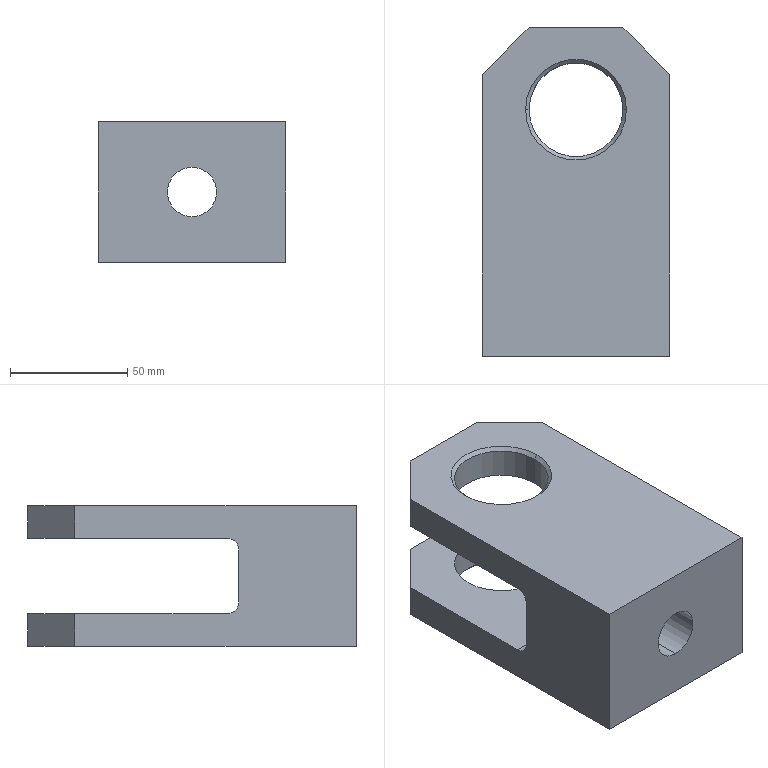Part | SolidWorks | features Chamfer 2, ICE 2, Extrusion 1, Fillet 1, HoleWzd 1 | 1 solid | 26 faces | box 80 x 140 x 60 mm | volume 378465 mm3 | plane 14 | cylinder 8 | cone 4 | commonest cylinder face diameters 40 x4 10 x2 21 x2
STEP:
#1=CARTESIAN_POINT('',(0.,-70.,-10.5));
#2=VERTEX_POINT('',#1);
#3=CARTESIAN_POINT('',(0.,-70.,10.5));
#4=VERTEX_POINT('',#3);
#5=CARTESIAN_POINT('',(0.,-70.,0.));
#6=DIRECTION('',(0.,1.,0.));
#7=DIRECTION('',(0.,0.,1.));
#8=AXIS2_PLACEMENT_3D('',#5,#6,#7);
#9=CIRCLE('',#8,10.5);
#10=EDGE_CURVE('',#2,#4,#9,.T.);
#11=ORIENTED_EDGE('',*,*,#10,.F.);
#12=CARTESIAN_POINT('',(0.,-20.,-10.5));
#13=VERTEX_POINT('',#12);
#14=CARTESIAN_POINT('',(0.,-20.,-10.5));
#15=DIRECTION('',(0.,1.,0.));
#16=VECTOR('',#15,1000.);
#17=LINE('',#14,#16);
#18=EDGE_CURVE('',#2,#13,#17,.T.);
#19=ORIENTED_EDGE('',*,*,#18,.T.);
#20=CARTESIAN_POINT('',(0.,-20.,10.5));
#21=VERTEX_POINT('',#20);
#22=CARTESIAN_POINT('',(0.,-20.,0.));
#23=DIRECTION('',(0.,1.,0.));
#24=DIRECTION('',(0.,0.,1.));
#25=AXIS2_PLACEMENT_3D('',#22,#23,#24);
#26=CIRCLE('',#25,10.5);
#27=EDGE_CURVE('',#13,#21,#26,.T.);
#28=ORIENTED_EDGE('',*,*,#27,.T.);
#29=CARTESIAN_POINT('',(0.,-20.,10.5));
#30=DIRECTION('',(0.,1.,0.));
#31=VECTOR('',#30,1000.);
#32=LINE('',#29,#31);
#33=EDGE_CURVE('',#4,#21,#32,.T.);
#34=ORIENTED_EDGE('',*,*,#33,.F.);
#35=EDGE_LOOP('',(#11,#19,#28,#34));
#36=FACE_OUTER_BOUND('',#35,.T.);
#37=CARTESIAN_POINT('',(0.,-20.,0.));
#38=DIRECTION('',(0.,1.,0.));
#39=DIRECTION('',(0.,0.,1.));
#40=AXIS2_PLACEMENT_3D('',#37,#38,#39);
#41=CYLINDRICAL_SURFACE('',#40,10.5);
#42=ADVANCED_FACE('',(#36),#41,.F.);
#43=CARTESIAN_POINT('',(-20.,35.,28.5));
#44=VERTEX_POINT('',#43);
#45=CARTESIAN_POINT('',(20.,35.,28.5));
#46=VERTEX_POINT('',#45);
#47=CARTESIAN_POINT('',(0.,35.,28.5));
#48=DIRECTION('',(0.,0.,1.));
#49=DIRECTION('',(1.,0.,0.));
#50=AXIS2_PLACEMENT_3D('',#47,#48,#49);
#51=CIRCLE('',#50,20.);
#52=EDGE_CURVE('',#44,#46,#51,.T.);
#53=ORIENTED_EDGE('',*,*,#52,.F.);
#54=CARTESIAN_POINT('',(-21.5,35.,30.));
#55=VERTEX_POINT('',#54);
#56=CARTESIAN_POINT('',(-20.,35.,28.5));
#57=DIRECTION('',(-0.7071,0.,0.7071));
#58=VECTOR('',#57,1000.);
#59=LINE('',#56,#58);
#60=EDGE_CURVE('',#44,#55,#59,.T.);
#61=ORIENTED_EDGE('',*,*,#60,.T.);
#62=CARTESIAN_POINT('',(21.5,35.,30.));
#63=VERTEX_POINT('',#62);
#64=CARTESIAN_POINT('',(0.,35.,30.));
#65=DIRECTION('',(0.,0.,-1.));
#66=DIRECTION('',(1.,0.,0.));
#67=AXIS2_PLACEMENT_3D('',#64,#65,#66);
#68=CIRCLE('',#67,21.5);
#69=EDGE_CURVE('',#63,#55,#68,.T.);
#70=ORIENTED_EDGE('',*,*,#69,.F.);
#71=CARTESIAN_POINT('',(20.,35.,28.5));
#72=DIRECTION('',(0.7071,0.,0.7071));
#73=VECTOR('',#72,1000.);
#74=LINE('',#71,#73);
#75=EDGE_CURVE('',#46,#63,#74,.T.);
#76=ORIENTED_EDGE('',*,*,#75,.F.);
#77=EDGE_LOOP('',(#53,#61,#70,#76));
#78=FACE_OUTER_BOUND('',#77,.T.);
#79=CARTESIAN_POINT('',(0.,35.,28.5));
#80=DIRECTION('',(0.,0.,1.));
#81=DIRECTION('',(1.,0.,0.));
#82=AXIS2_PLACEMENT_3D('',#79,#80,#81);
#83=CONICAL_SURFACE('',#82,20.,0.7854);
#84=ADVANCED_FACE('',(#78),#83,.F.);
#85=CARTESIAN_POINT('',(20.,35.,-28.5));
#86=VERTEX_POINT('',#85);
#87=CARTESIAN_POINT('',(-20.,35.,-28.5));
#88=VERTEX_POINT('',#87);
#89=CARTESIAN_POINT('',(0.,35.,-28.5));
#90=DIRECTION('',(0.,0.,-1.));
#91=DIRECTION('',(1.,0.,0.));
#92=AXIS2_PLACEMENT_3D('',#89,#90,#91);
#93=CIRCLE('',#92,20.);
#94=EDGE_CURVE('',#86,#88,#93,.T.);
#95=ORIENTED_EDGE('',*,*,#94,.F.);
#96=CARTESIAN_POINT('',(21.5,35.,-30.));
#97=VERTEX_POINT('',#96);
#98=CARTESIAN_POINT('',(21.5,35.,-30.));
#99=DIRECTION('',(0.7071,0.,-0.7071));
#100=VECTOR('',#99,1000.);
#101=LINE('',#98,#100);
#102=EDGE_CURVE('',#86,#97,#101,.T.);
#103=ORIENTED_EDGE('',*,*,#102,.T.);
#104=CARTESIAN_POINT('',(-21.5,35.,-30.));
#105=VERTEX_POINT('',#104);
#106=CARTESIAN_POINT('',(0.,35.,-30.));
#107=DIRECTION('',(0.,0.,1.));
#108=DIRECTION('',(1.,0.,0.));
#109=AXIS2_PLACEMENT_3D('',#106,#107,#108);
#110=CIRCLE('',#109,21.5);
#111=EDGE_CURVE('',#105,#97,#110,.T.);
#112=ORIENTED_EDGE('',*,*,#111,.F.);
#113=CARTESIAN_POINT('',(-21.5,35.,-30.));
#114=DIRECTION('',(-0.7071,0.,-0.7071));
#115=VECTOR('',#114,1000.);
#116=LINE('',#113,#115);
#117=EDGE_CURVE('',#88,#105,#116,.T.);
#118=ORIENTED_EDGE('',*,*,#117,.F.);
#119=EDGE_LOOP('',(#95,#103,#112,#118));
#120=FACE_OUTER_BOUND('',#119,.T.);
#121=CARTESIAN_POINT('',(0.,35.,-30.));
#122=DIRECTION('',(0.,0.,-1.));
#123=DIRECTION('',(-1.,0.,0.));
#124=AXIS2_PLACEMENT_3D('',#121,#122,#123);
#125=CONICAL_SURFACE('',#124,21.5,0.7854);
#126=ADVANCED_FACE('',(#120),#125,.F.);
#127=ORIENTED_EDGE('',*,*,#94,.T.);
#128=CARTESIAN_POINT('',(-20.,35.,-16.));
#129=VERTEX_POINT('',#128);
#130=CARTESIAN_POINT('',(-20.,35.,-30.));
#131=DIRECTION('',(0.,0.,1.));
#132=VECTOR('',#131,1000.);
#133=LINE('',#130,#132);
#134=EDGE_CURVE('',#88,#129,#133,.T.);
#135=ORIENTED_EDGE('',*,*,#134,.T.);
#136=CARTESIAN_POINT('',(20.,35.,-16.));
#137=VERTEX_POINT('',#136);
#138=CARTESIAN_POINT('',(0.,35.,-16.));
#139=DIRECTION('',(0.,0.,-1.));
#140=DIRECTION('',(-1.,0.,0.));
#141=AXIS2_PLACEMENT_3D('',#138,#139,#140);
#142=CIRCLE('',#141,20.);
#143=EDGE_CURVE('',#137,#129,#142,.T.);
#144=ORIENTED_EDGE('',*,*,#143,.F.);
#145=CARTESIAN_POINT('',(20.,35.,-30.));
#146=DIRECTION('',(0.,0.,1.));
#147=VECTOR('',#146,1000.);
#148=LINE('',#145,#147);
#149=EDGE_CURVE('',#86,#137,#148,.T.);
#150=ORIENTED_EDGE('',*,*,#149,.F.);
#151=EDGE_LOOP('',(#127,#135,#144,#150));
#152=FACE_OUTER_BOUND('',#151,.T.);
#153=CARTESIAN_POINT('',(0.,35.,-30.));
#154=DIRECTION('',(0.,0.,1.));
#155=DIRECTION('',(1.,0.,0.));
#156=AXIS2_PLACEMENT_3D('',#153,#154,#155);
#157=CYLINDRICAL_SURFACE('',#156,20.);
#158=ADVANCED_FACE('',(#152),#157,.F.);
#159=CARTESIAN_POINT('',(-20.,35.,16.));
#160=VERTEX_POINT('',#159);
#161=CARTESIAN_POINT('',(20.,35.,16.));
#162=VERTEX_POINT('',#161);
#163=CARTESIAN_POINT('',(0.,35.,16.));
#164=DIRECTION('',(0.,0.,1.));
#165=DIRECTION('',(0.,-1.,0.));
#166=AXIS2_PLACEMENT_3D('',#163,#164,#165);
#167=CIRCLE('',#166,20.);
#168=EDGE_CURVE('',#160,#162,#167,.T.);
#169=ORIENTED_EDGE('',*,*,#168,.F.);
#170=CARTESIAN_POINT('',(-20.,35.,-30.));
#171=DIRECTION('',(0.,0.,1.));
#172=VECTOR('',#171,1000.);
#173=LINE('',#170,#172);
#174=EDGE_CURVE('',#160,#44,#173,.T.);
#175=ORIENTED_EDGE('',*,*,#174,.T.);
#176=ORIENTED_EDGE('',*,*,#52,.T.);
#177=CARTESIAN_POINT('',(20.,35.,-30.));
#178=DIRECTION('',(0.,0.,1.));
#179=VECTOR('',#178,1000.);
#180=LINE('',#177,#179);
#181=EDGE_CURVE('',#162,#46,#180,.T.);
#182=ORIENTED_EDGE('',*,*,#181,.F.);
#183=EDGE_LOOP('',(#169,#175,#176,#182));
#184=FACE_OUTER_BOUND('',#183,.T.);
#185=CARTESIAN_POINT('',(0.,35.,-30.));
#186=DIRECTION('',(0.,0.,1.));
#187=DIRECTION('',(1.,0.,0.));
#188=AXIS2_PLACEMENT_3D('',#185,#186,#187);
#189=CYLINDRICAL_SURFACE('',#188,20.);
#190=ADVANCED_FACE('',(#184),#189,.F.);
#191=CARTESIAN_POINT('',(-20.,70.,-30.));
#192=VERTEX_POINT('',#191);
#193=CARTESIAN_POINT('',(-20.,70.,-16.));
#194=VERTEX_POINT('',#193);
#195=CARTESIAN_POINT('',(-20.,70.,30.));
#196=DIRECTION('',(0.,0.,1.));
#197=VECTOR('',#196,1000.);
#198=LINE('',#195,#197);
#199=EDGE_CURVE('',#192,#194,#198,.T.);
#200=ORIENTED_EDGE('',*,*,#199,.T.);
#201=CARTESIAN_POINT('',(20.,70.,-16.));
#202=VERTEX_POINT('',#201);
#203=CARTESIAN_POINT('',(40.,70.,-16.));
#204=DIRECTION('',(1.,0.,0.));
#205=VECTOR('',#204,1000.);
#206=LINE('',#203,#205);
#207=EDGE_CURVE('',#194,#202,#206,.T.);
#208=ORIENTED_EDGE('',*,*,#207,.T.);
#209=CARTESIAN_POINT('',(20.,70.,-30.));
#210=VERTEX_POINT('',#209);
#211=CARTESIAN_POINT('',(20.,70.,30.));
#212=DIRECTION('',(0.,0.,-1.));
#213=VECTOR('',#212,1000.);
#214=LINE('',#211,#213);
#215=EDGE_CURVE('',#202,#210,#214,.T.);
#216=ORIENTED_EDGE('',*,*,#215,.T.);
#217=CARTESIAN_POINT('',(40.,70.,-30.));
#218=DIRECTION('',(-1.,0.,0.));
#219=VECTOR('',#218,1000.);
#220=LINE('',#217,#219);
#221=EDGE_CURVE('',#210,#192,#220,.T.);
#222=ORIENTED_EDGE('',*,*,#221,.T.);
#223=EDGE_LOOP('',(#200,#208,#216,#222));
#224=FACE_OUTER_BOUND('',#223,.T.);
#225=CARTESIAN_POINT('',(40.,70.,30.));
#226=DIRECTION('',(0.,-1.,0.));
#227=DIRECTION('',(0.,0.,-1.));
#228=AXIS2_PLACEMENT_3D('',#225,#226,#227);
#229=PLANE('',#228);
#230=ADVANCED_FACE('',(#224),#229,.F.);
#231=CARTESIAN_POINT('',(40.,50.,-16.));
#232=VERTEX_POINT('',#231);
#233=CARTESIAN_POINT('',(20.,70.,-16.));
#234=DIRECTION('',(-0.7071,0.7071,0.));
#235=VECTOR('',#234,1000.);
#236=LINE('',#233,#235);
#237=EDGE_CURVE('',#232,#202,#236,.T.);
#238=ORIENTED_EDGE('',*,*,#237,.F.);
#239=CARTESIAN_POINT('',(40.,50.,-30.));
#240=VERTEX_POINT('',#239);
#241=CARTESIAN_POINT('',(40.,50.,30.));
#242=DIRECTION('',(0.,0.,1.));
#243=VECTOR('',#242,1000.);
#244=LINE('',#241,#243);
#245=EDGE_CURVE('',#240,#232,#244,.T.);
#246=ORIENTED_EDGE('',*,*,#245,.F.);
#247=CARTESIAN_POINT('',(20.,70.,-30.));
#248=DIRECTION('',(0.7071,-0.7071,0.));
#249=VECTOR('',#248,1000.);
#250=LINE('',#247,#249);
#251=EDGE_CURVE('',#210,#240,#250,.T.);
#252=ORIENTED_EDGE('',*,*,#251,.F.);
#253=ORIENTED_EDGE('',*,*,#215,.F.);
#254=EDGE_LOOP('',(#238,#246,#252,#253));
#255=FACE_OUTER_BOUND('',#254,.T.);
#256=CARTESIAN_POINT('',(20.,70.,30.));
#257=DIRECTION('',(-0.7071,-0.7071,0.));
#258=DIRECTION('',(0.,0.,-1.));
#259=AXIS2_PLACEMENT_3D('',#256,#257,#258);
#260=PLANE('',#259);
#261=ADVANCED_FACE('',(#255),#260,.F.);
#262=CARTESIAN_POINT('',(-40.,50.,-16.));
#263=VERTEX_POINT('',#262);
#264=CARTESIAN_POINT('',(-40.,50.,-16.));
#265=DIRECTION('',(-0.7071,-0.7071,0.));
#266=VECTOR('',#265,1000.);
#267=LINE('',#264,#266);
#268=EDGE_CURVE('',#194,#263,#267,.T.);
#269=ORIENTED_EDGE('',*,*,#268,.F.);
#270=ORIENTED_EDGE('',*,*,#199,.F.);
#271=CARTESIAN_POINT('',(-40.,50.,-30.));
#272=VERTEX_POINT('',#271);
#273=CARTESIAN_POINT('',(-40.,50.,-30.));
#274=DIRECTION('',(0.7071,0.7071,0.));
#275=VECTOR('',#274,1000.);
#276=LINE('',#273,#275);
#277=EDGE_CURVE('',#272,#192,#276,.T.);
#278=ORIENTED_EDGE('',*,*,#277,.F.);
#279=CARTESIAN_POINT('',(-40.,50.,30.));
#280=DIRECTION('',(0.,0.,-1.));
#281=VECTOR('',#280,1000.);
#282=LINE('',#279,#281);
#283=EDGE_CURVE('',#263,#272,#282,.T.);
#284=ORIENTED_EDGE('',*,*,#283,.F.);
#285=EDGE_LOOP('',(#269,#270,#278,#284));
#286=FACE_OUTER_BOUND('',#285,.T.);
#287=CARTESIAN_POINT('',(-40.,50.,30.));
#288=DIRECTION('',(0.7071,-0.7071,0.));
#289=DIRECTION('',(0.,0.,-1.));
#290=AXIS2_PLACEMENT_3D('',#287,#288,#289);
#291=PLANE('',#290);
#292=ADVANCED_FACE('',(#286),#291,.F.);
#293=CARTESIAN_POINT('',(-40.,50.,16.));
#294=VERTEX_POINT('',#293);
#295=CARTESIAN_POINT('',(-40.,-15.,16.));
#296=VERTEX_POINT('',#295);
#297=CARTESIAN_POINT('',(-40.,-70.,16.));
#298=DIRECTION('',(0.,-1.,0.));
#299=VECTOR('',#298,1000.);
#300=LINE('',#297,#299);
#301=EDGE_CURVE('',#294,#296,#300,.T.);
#302=ORIENTED_EDGE('',*,*,#301,.T.);
#303=CARTESIAN_POINT('',(-40.,-20.,11.));
#304=VERTEX_POINT('',#303);
#305=CARTESIAN_POINT('',(-40.,-15.,11.));
#306=DIRECTION('',(1.,0.,0.));
#307=DIRECTION('',(0.,1.,0.));
#308=AXIS2_PLACEMENT_3D('',#305,#306,#307);
#309=CIRCLE('',#308,5.);
#310=EDGE_CURVE('',#296,#304,#309,.T.);
#311=ORIENTED_EDGE('',*,*,#310,.T.);
#312=CARTESIAN_POINT('',(-40.,-20.,-11.));
#313=VERTEX_POINT('',#312);
#314=CARTESIAN_POINT('',(-40.,-20.,30.));
#315=DIRECTION('',(0.,0.,-1.));
#316=VECTOR('',#315,1000.);
#317=LINE('',#314,#316);
#318=EDGE_CURVE('',#304,#313,#317,.T.);
#319=ORIENTED_EDGE('',*,*,#318,.T.);
#320=CARTESIAN_POINT('',(-40.,-15.,-16.));
#321=VERTEX_POINT('',#320);
#322=CARTESIAN_POINT('',(-40.,-15.,-11.));
#323=DIRECTION('',(1.,0.,0.));
#324=DIRECTION('',(0.,1.,0.));
#325=AXIS2_PLACEMENT_3D('',#322,#323,#324);
#326=CIRCLE('',#325,5.);
#327=EDGE_CURVE('',#313,#321,#326,.T.);
#328=ORIENTED_EDGE('',*,*,#327,.T.);
#329=CARTESIAN_POINT('',(-40.,-70.,-16.));
#330=DIRECTION('',(0.,1.,0.));
#331=VECTOR('',#330,1000.);
#332=LINE('',#329,#331);
#333=EDGE_CURVE('',#321,#263,#332,.T.);
#334=ORIENTED_EDGE('',*,*,#333,.T.);
#335=ORIENTED_EDGE('',*,*,#283,.T.);
#336=CARTESIAN_POINT('',(-40.,-70.,-30.));
#337=VERTEX_POINT('',#336);
#338=CARTESIAN_POINT('',(-40.,-70.,-30.));
#339=DIRECTION('',(0.,-1.,0.));
#340=VECTOR('',#339,1000.);
#341=LINE('',#338,#340);
#342=EDGE_CURVE('',#272,#337,#341,.T.);
#343=ORIENTED_EDGE('',*,*,#342,.T.);
#344=CARTESIAN_POINT('',(-40.,-70.,30.));
#345=VERTEX_POINT('',#344);
#346=CARTESIAN_POINT('',(-40.,-70.,30.));
#347=DIRECTION('',(0.,0.,-1.));
#348=VECTOR('',#347,1000.);
#349=LINE('',#346,#348);
#350=EDGE_CURVE('',#345,#337,#349,.T.);
#351=ORIENTED_EDGE('',*,*,#350,.F.);
#352=CARTESIAN_POINT('',(-40.,50.,30.));
#353=VERTEX_POINT('',#352);
#354=CARTESIAN_POINT('',(-40.,-70.,30.));
#355=DIRECTION('',(0.,-1.,0.));
#356=VECTOR('',#355,1000.);
#357=LINE('',#354,#356);
#358=EDGE_CURVE('',#353,#345,#357,.T.);
#359=ORIENTED_EDGE('',*,*,#358,.F.);
#360=CARTESIAN_POINT('',(-40.,50.,30.));
#361=DIRECTION('',(0.,0.,-1.));
#362=VECTOR('',#361,1000.);
#363=LINE('',#360,#362);
#364=EDGE_CURVE('',#353,#294,#363,.T.);
#365=ORIENTED_EDGE('',*,*,#364,.T.);
#366=EDGE_LOOP('',(#302,#311,#319,#328,#334,#335,#343,#351,#359,#365));
#367=FACE_OUTER_BOUND('',#366,.T.);
#368=CARTESIAN_POINT('',(-40.,-70.,30.));
#369=DIRECTION('',(1.,0.,0.));
#370=DIRECTION('',(0.,1.,0.));
#371=AXIS2_PLACEMENT_3D('',#368,#369,#370);
#372=PLANE('',#371);
#373=ADVANCED_FACE('',(#367),#372,.F.);
#374=CARTESIAN_POINT('',(0.,-70.,0.));
#375=DIRECTION('',(0.,1.,0.));
#376=DIRECTION('',(0.,0.,1.));
#377=AXIS2_PLACEMENT_3D('',#374,#375,#376);
#378=CIRCLE('',#377,10.5);
#379=EDGE_CURVE('',#4,#2,#378,.T.);
#380=ORIENTED_EDGE('',*,*,#379,.T.);
#381=ORIENTED_EDGE('',*,*,#10,.T.);
#382=EDGE_LOOP('',(#380,#381));
#383=FACE_BOUND('',#382,.T.);
#384=CARTESIAN_POINT('',(40.,-70.,-30.));
#385=VERTEX_POINT('',#384);
#386=CARTESIAN_POINT('',(40.,-70.,-30.));
#387=DIRECTION('',(1.,0.,0.));
#388=VECTOR('',#387,1000.);
#389=LINE('',#386,#388);
#390=EDGE_CURVE('',#337,#385,#389,.T.);
#391=ORIENTED_EDGE('',*,*,#390,.T.);
#392=CARTESIAN_POINT('',(40.,-70.,30.));
#393=VERTEX_POINT('',#392);
#394=CARTESIAN_POINT('',(40.,-70.,30.));
#395=DIRECTION('',(0.,0.,-1.));
#396=VECTOR('',#395,1000.);
#397=LINE('',#394,#396);
#398=EDGE_CURVE('',#393,#385,#397,.T.);
#399=ORIENTED_EDGE('',*,*,#398,.F.);
#400=CARTESIAN_POINT('',(40.,-70.,30.));
#401=DIRECTION('',(1.,0.,0.));
#402=VECTOR('',#401,1000.);
#403=LINE('',#400,#402);
#404=EDGE_CURVE('',#345,#393,#403,.T.);
#405=ORIENTED_EDGE('',*,*,#404,.F.);
#406=ORIENTED_EDGE('',*,*,#350,.T.);
#407=EDGE_LOOP('',(#391,#399,#405,#406));
#408=FACE_OUTER_BOUND('',#407,.T.);
#409=CARTESIAN_POINT('',(40.,-70.,30.));
#410=DIRECTION('',(0.,1.,0.));
#411=DIRECTION('',(0.,0.,1.));
#412=AXIS2_PLACEMENT_3D('',#409,#410,#411);
#413=PLANE('',#412);
#414=ADVANCED_FACE('',(#383,#408),#413,.F.);
#415=ORIENTED_EDGE('',*,*,#245,.T.);
#416=CARTESIAN_POINT('',(40.,-15.,-16.));
#417=VERTEX_POINT('',#416);
#418=CARTESIAN_POINT('',(40.,160.,-16.));
#419=DIRECTION('',(0.,-1.,0.));
#420=VECTOR('',#419,1000.);
#421=LINE('',#418,#420);
#422=EDGE_CURVE('',#232,#417,#421,.T.);
#423=ORIENTED_EDGE('',*,*,#422,.T.);
#424=CARTESIAN_POINT('',(40.,-20.,-11.));
#425=VERTEX_POINT('',#424);
#426=CARTESIAN_POINT('',(40.,-15.,-11.));
#427=DIRECTION('',(-1.,0.,0.));
#428=DIRECTION('',(0.,-1.,0.));
#429=AXIS2_PLACEMENT_3D('',#426,#427,#428);
#430=CIRCLE('',#429,5.);
#431=EDGE_CURVE('',#417,#425,#430,.T.);
#432=ORIENTED_EDGE('',*,*,#431,.T.);
#433=CARTESIAN_POINT('',(40.,-20.,11.));
#434=VERTEX_POINT('',#433);
#435=CARTESIAN_POINT('',(40.,-20.,16.));
#436=DIRECTION('',(0.,0.,1.));
#437=VECTOR('',#436,1000.);
#438=LINE('',#435,#437);
#439=EDGE_CURVE('',#425,#434,#438,.T.);
#440=ORIENTED_EDGE('',*,*,#439,.T.);
#441=CARTESIAN_POINT('',(40.,-15.,16.));
#442=VERTEX_POINT('',#441);
#443=CARTESIAN_POINT('',(40.,-15.,11.));
#444=DIRECTION('',(-1.,0.,0.));
#445=DIRECTION('',(0.,-1.,0.));
#446=AXIS2_PLACEMENT_3D('',#443,#444,#445);
#447=CIRCLE('',#446,5.);
#448=EDGE_CURVE('',#434,#442,#447,.T.);
#449=ORIENTED_EDGE('',*,*,#448,.T.);
#450=CARTESIAN_POINT('',(40.,50.,16.));
#451=VERTEX_POINT('',#450);
#452=CARTESIAN_POINT('',(40.,160.,16.));
#453=DIRECTION('',(0.,1.,0.));
#454=VECTOR('',#453,1000.);
#455=LINE('',#452,#454);
#456=EDGE_CURVE('',#442,#451,#455,.T.);
#457=ORIENTED_EDGE('',*,*,#456,.T.);
#458=CARTESIAN_POINT('',(40.,50.,30.));
#459=VERTEX_POINT('',#458);
#460=CARTESIAN_POINT('',(40.,50.,30.));
#461=DIRECTION('',(0.,0.,1.));
#462=VECTOR('',#461,1000.);
#463=LINE('',#460,#462);
#464=EDGE_CURVE('',#451,#459,#463,.T.);
#465=ORIENTED_EDGE('',*,*,#464,.T.);
#466=CARTESIAN_POINT('',(40.,-70.,30.));
#467=DIRECTION('',(0.,1.,0.));
#468=VECTOR('',#467,1000.);
#469=LINE('',#466,#468);
#470=EDGE_CURVE('',#393,#459,#469,.T.);
#471=ORIENTED_EDGE('',*,*,#470,.F.);
#472=ORIENTED_EDGE('',*,*,#398,.T.);
#473=CARTESIAN_POINT('',(40.,-70.,-30.));
#474=DIRECTION('',(0.,1.,0.));
#475=VECTOR('',#474,1000.);
#476=LINE('',#473,#475);
#477=EDGE_CURVE('',#385,#240,#476,.T.);
#478=ORIENTED_EDGE('',*,*,#477,.T.);
#479=EDGE_LOOP('',(#415,#423,#432,#440,#449,#457,#465,#471,#472,#478));
#480=FACE_OUTER_BOUND('',#479,.T.);
#481=CARTESIAN_POINT('',(40.,-70.,30.));
#482=DIRECTION('',(-1.,0.,0.));
#483=DIRECTION('',(0.,-1.,0.));
#484=AXIS2_PLACEMENT_3D('',#481,#482,#483);
#485=PLANE('',#484);
#486=ADVANCED_FACE('',(#480),#485,.F.);
#487=CARTESIAN_POINT('',(20.,70.,30.));
#488=VERTEX_POINT('',#487);
#489=CARTESIAN_POINT('',(20.,70.,16.));
#490=VERTEX_POINT('',#489);
#491=CARTESIAN_POINT('',(20.,70.,30.));
#492=DIRECTION('',(0.,0.,-1.));
#493=VECTOR('',#492,1000.);
#494=LINE('',#491,#493);
#495=EDGE_CURVE('',#488,#490,#494,.T.);
#496=ORIENTED_EDGE('',*,*,#495,.T.);
#497=CARTESIAN_POINT('',(-20.,70.,16.));
#498=VERTEX_POINT('',#497);
#499=CARTESIAN_POINT('',(40.,70.,16.));
#500=DIRECTION('',(-1.,0.,0.));
#501=VECTOR('',#500,1000.);
#502=LINE('',#499,#501);
#503=EDGE_CURVE('',#490,#498,#502,.T.);
#504=ORIENTED_EDGE('',*,*,#503,.T.);
#505=CARTESIAN_POINT('',(-20.,70.,30.));
#506=VERTEX_POINT('',#505);
#507=CARTESIAN_POINT('',(-20.,70.,30.));
#508=DIRECTION('',(0.,0.,1.));
#509=VECTOR('',#508,1000.);
#510=LINE('',#507,#509);
#511=EDGE_CURVE('',#498,#506,#510,.T.);
#512=ORIENTED_EDGE('',*,*,#511,.T.);
#513=CARTESIAN_POINT('',(40.,70.,30.));
#514=DIRECTION('',(-1.,0.,0.));
#515=VECTOR('',#514,1000.);
#516=LINE('',#513,#515);
#517=EDGE_CURVE('',#488,#506,#516,.T.);
#518=ORIENTED_EDGE('',*,*,#517,.F.);
#519=EDGE_LOOP('',(#496,#504,#512,#518));
#520=FACE_OUTER_BOUND('',#519,.T.);
#521=CARTESIAN_POINT('',(40.,70.,30.));
#522=DIRECTION('',(0.,-1.,0.));
#523=DIRECTION('',(0.,0.,-1.));
#524=AXIS2_PLACEMENT_3D('',#521,#522,#523);
#525=PLANE('',#524);
#526=ADVANCED_FACE('',(#520),#525,.F.);
#527=ORIENTED_EDGE('',*,*,#69,.T.);
#528=CARTESIAN_POINT('',(0.,35.,30.));
#529=DIRECTION('',(0.,0.,-1.));
#530=DIRECTION('',(1.,0.,0.));
#531=AXIS2_PLACEMENT_3D('',#528,#529,#530);
#532=CIRCLE('',#531,21.5);
#533=EDGE_CURVE('',#55,#63,#532,.T.);
#534=ORIENTED_EDGE('',*,*,#533,.T.);
#535=EDGE_LOOP('',(#527,#534));
#536=FACE_BOUND('',#535,.T.);
#537=ORIENTED_EDGE('',*,*,#470,.T.);
#538=CARTESIAN_POINT('',(45.,45.,30.));
#539=DIRECTION('',(-0.7071,0.7071,0.));
#540=VECTOR('',#539,1000.);
#541=LINE('',#538,#540);
#542=EDGE_CURVE('',#459,#488,#541,.T.);
#543=ORIENTED_EDGE('',*,*,#542,.T.);
#544=ORIENTED_EDGE('',*,*,#517,.T.);
#545=CARTESIAN_POINT('',(-45.,45.,30.));
#546=DIRECTION('',(-0.7071,-0.7071,0.));
#547=VECTOR('',#546,1000.);
#548=LINE('',#545,#547);
#549=EDGE_CURVE('',#506,#353,#548,.T.);
#550=ORIENTED_EDGE('',*,*,#549,.T.);
#551=ORIENTED_EDGE('',*,*,#358,.T.);
#552=ORIENTED_EDGE('',*,*,#404,.T.);
#553=EDGE_LOOP('',(#537,#543,#544,#550,#551,#552));
#554=FACE_OUTER_BOUND('',#553,.T.);
#555=CARTESIAN_POINT('',(0.,0.,30.));
#556=DIRECTION('',(0.,0.,1.));
#557=DIRECTION('',(1.,0.,0.));
#558=AXIS2_PLACEMENT_3D('',#555,#556,#557);
#559=PLANE('',#558);
#560=ADVANCED_FACE('',(#536,#554),#559,.T.);
#561=ORIENTED_EDGE('',*,*,#111,.T.);
#562=CARTESIAN_POINT('',(0.,35.,-30.));
#563=DIRECTION('',(0.,0.,1.));
#564=DIRECTION('',(1.,0.,0.));
#565=AXIS2_PLACEMENT_3D('',#562,#563,#564);
#566=CIRCLE('',#565,21.5);
#567=EDGE_CURVE('',#97,#105,#566,.T.);
#568=ORIENTED_EDGE('',*,*,#567,.T.);
#569=EDGE_LOOP('',(#561,#568));
#570=FACE_BOUND('',#569,.T.);
#571=ORIENTED_EDGE('',*,*,#221,.F.);
#572=ORIENTED_EDGE('',*,*,#251,.T.);
#573=ORIENTED_EDGE('',*,*,#477,.F.);
#574=ORIENTED_EDGE('',*,*,#390,.F.);
#575=ORIENTED_EDGE('',*,*,#342,.F.);
#576=ORIENTED_EDGE('',*,*,#277,.T.);
#577=EDGE_LOOP('',(#571,#572,#573,#574,#575,#576));
#578=FACE_OUTER_BOUND('',#577,.T.);
#579=CARTESIAN_POINT('',(0.,0.,-30.));
#580=DIRECTION('',(0.,0.,1.));
#581=DIRECTION('',(1.,0.,0.));
#582=AXIS2_PLACEMENT_3D('',#579,#580,#581);
#583=PLANE('',#582);
#584=ADVANCED_FACE('',(#570,#578),#583,.F.);
#585=CARTESIAN_POINT('',(20.,70.,16.));
#586=DIRECTION('',(0.7071,-0.7071,0.));
#587=VECTOR('',#586,1000.);
#588=LINE('',#585,#587);
#589=EDGE_CURVE('',#490,#451,#588,.T.);
#590=ORIENTED_EDGE('',*,*,#589,.F.);
#591=ORIENTED_EDGE('',*,*,#495,.F.);
#592=ORIENTED_EDGE('',*,*,#542,.F.);
#593=ORIENTED_EDGE('',*,*,#464,.F.);
#594=EDGE_LOOP('',(#590,#591,#592,#593));
#595=FACE_OUTER_BOUND('',#594,.T.);
#596=CARTESIAN_POINT('',(20.,70.,30.));
#597=DIRECTION('',(-0.7071,-0.7071,0.));
#598=DIRECTION('',(0.,0.,-1.));
#599=AXIS2_PLACEMENT_3D('',#596,#597,#598);
#600=PLANE('',#599);
#601=ADVANCED_FACE('',(#595),#600,.F.);
#602=CARTESIAN_POINT('',(-40.,50.,16.));
#603=DIRECTION('',(0.7071,0.7071,0.));
#604=VECTOR('',#603,1000.);
#605=LINE('',#602,#604);
#606=EDGE_CURVE('',#294,#498,#605,.T.);
#607=ORIENTED_EDGE('',*,*,#606,.F.);
#608=ORIENTED_EDGE('',*,*,#364,.F.);
#609=ORIENTED_EDGE('',*,*,#549,.F.);
#610=ORIENTED_EDGE('',*,*,#511,.F.);
#611=EDGE_LOOP('',(#607,#608,#609,#610));
#612=FACE_OUTER_BOUND('',#611,.T.);
#613=CARTESIAN_POINT('',(-40.,50.,30.));
#614=DIRECTION('',(0.7071,-0.7071,0.));
#615=DIRECTION('',(0.,0.,-1.));
#616=AXIS2_PLACEMENT_3D('',#613,#614,#615);
#617=PLANE('',#616);
#618=ADVANCED_FACE('',(#612),#617,.F.);
#619=CARTESIAN_POINT('',(0.,-20.,0.));
#620=DIRECTION('',(0.,1.,0.));
#621=DIRECTION('',(0.,0.,1.));
#622=AXIS2_PLACEMENT_3D('',#619,#620,#621);
#623=CIRCLE('',#622,10.5);
#624=EDGE_CURVE('',#21,#13,#623,.T.);
#625=ORIENTED_EDGE('',*,*,#624,.F.);
#626=ORIENTED_EDGE('',*,*,#27,.F.);
#627=EDGE_LOOP('',(#625,#626));
#628=FACE_BOUND('',#627,.T.);
#629=ORIENTED_EDGE('',*,*,#318,.F.);
#630=CARTESIAN_POINT('',(40.,-20.,11.));
#631=DIRECTION('',(1.,0.,0.));
#632=VECTOR('',#631,1000.);
#633=LINE('',#630,#632);
#634=EDGE_CURVE('',#304,#434,#633,.T.);
#635=ORIENTED_EDGE('',*,*,#634,.T.);
#636=ORIENTED_EDGE('',*,*,#439,.F.);
#637=CARTESIAN_POINT('',(-40.,-20.,-11.));
#638=DIRECTION('',(-1.,0.,0.));
#639=VECTOR('',#638,1000.);
#640=LINE('',#637,#639);
#641=EDGE_CURVE('',#425,#313,#640,.T.);
#642=ORIENTED_EDGE('',*,*,#641,.T.);
#643=EDGE_LOOP('',(#629,#635,#636,#642));
#644=FACE_OUTER_BOUND('',#643,.T.);
#645=CARTESIAN_POINT('',(40.,-20.,16.));
#646=DIRECTION('',(0.,-1.,0.));
#647=DIRECTION('',(1.,0.,0.));
#648=AXIS2_PLACEMENT_3D('',#645,#646,#647);
#649=PLANE('',#648);
#650=ADVANCED_FACE('',(#628,#644),#649,.F.);
#651=ORIENTED_EDGE('',*,*,#143,.T.);
#652=CARTESIAN_POINT('',(0.,35.,-16.));
#653=DIRECTION('',(0.,0.,-1.));
#654=DIRECTION('',(-1.,0.,0.));
#655=AXIS2_PLACEMENT_3D('',#652,#653,#654);
#656=CIRCLE('',#655,20.);
#657=EDGE_CURVE('',#129,#137,#656,.T.);
#658=ORIENTED_EDGE('',*,*,#657,.T.);
#659=EDGE_LOOP('',(#651,#658));
#660=FACE_BOUND('',#659,.T.);
#661=ORIENTED_EDGE('',*,*,#333,.F.);
#662=CARTESIAN_POINT('',(40.,-15.,-16.));
#663=DIRECTION('',(1.,0.,0.));
#664=VECTOR('',#663,1000.);
#665=LINE('',#662,#664);
#666=EDGE_CURVE('',#321,#417,#665,.T.);
#667=ORIENTED_EDGE('',*,*,#666,.T.);
#668=ORIENTED_EDGE('',*,*,#422,.F.);
#669=ORIENTED_EDGE('',*,*,#237,.T.);
#670=ORIENTED_EDGE('',*,*,#207,.F.);
#671=ORIENTED_EDGE('',*,*,#268,.T.);
#672=EDGE_LOOP('',(#661,#667,#668,#669,#670,#671));
#673=FACE_OUTER_BOUND('',#672,.T.);
#674=CARTESIAN_POINT('',(40.,160.,-16.));
#675=DIRECTION('',(0.,0.,-1.));
#676=DIRECTION('',(-1.,0.,0.));
#677=AXIS2_PLACEMENT_3D('',#674,#675,#676);
#678=PLANE('',#677);
#679=ADVANCED_FACE('',(#660,#673),#678,.F.);
#680=CARTESIAN_POINT('',(0.,35.,16.));
#681=DIRECTION('',(0.,0.,1.));
#682=DIRECTION('',(0.,-1.,0.));
#683=AXIS2_PLACEMENT_3D('',#680,#681,#682);
#684=CIRCLE('',#683,20.);
#685=EDGE_CURVE('',#162,#160,#684,.T.);
#686=ORIENTED_EDGE('',*,*,#685,.T.);
#687=ORIENTED_EDGE('',*,*,#168,.T.);
#688=EDGE_LOOP('',(#686,#687));
#689=FACE_BOUND('',#688,.T.);
#690=ORIENTED_EDGE('',*,*,#456,.F.);
#691=CARTESIAN_POINT('',(-40.,-15.,16.));
#692=DIRECTION('',(-1.,0.,0.));
#693=VECTOR('',#692,1000.);
#694=LINE('',#691,#693);
#695=EDGE_CURVE('',#442,#296,#694,.T.);
#696=ORIENTED_EDGE('',*,*,#695,.T.);
#697=ORIENTED_EDGE('',*,*,#301,.F.);
#698=ORIENTED_EDGE('',*,*,#606,.T.);
#699=ORIENTED_EDGE('',*,*,#503,.F.);
#700=ORIENTED_EDGE('',*,*,#589,.T.);
#701=EDGE_LOOP('',(#690,#696,#697,#698,#699,#700));
#702=FACE_OUTER_BOUND('',#701,.T.);
#703=CARTESIAN_POINT('',(40.,160.,16.));
#704=DIRECTION('',(0.,0.,1.));
#705=DIRECTION('',(0.,-1.,0.));
#706=AXIS2_PLACEMENT_3D('',#703,#704,#705);
#707=PLANE('',#706);
#708=ADVANCED_FACE('',(#689,#702),#707,.F.);
#709=ORIENTED_EDGE('',*,*,#448,.F.);
#710=ORIENTED_EDGE('',*,*,#634,.F.);
#711=ORIENTED_EDGE('',*,*,#310,.F.);
#712=ORIENTED_EDGE('',*,*,#695,.F.);
#713=EDGE_LOOP('',(#709,#710,#711,#712));
#714=FACE_OUTER_BOUND('',#713,.T.);
#715=CARTESIAN_POINT('',(40.,-15.,11.));
#716=DIRECTION('',(1.,0.,0.));
#717=DIRECTION('',(0.,1.,0.));
#718=AXIS2_PLACEMENT_3D('',#715,#716,#717);
#719=CYLINDRICAL_SURFACE('',#718,5.);
#720=ADVANCED_FACE('',(#714),#719,.F.);
#721=ORIENTED_EDGE('',*,*,#431,.F.);
#722=ORIENTED_EDGE('',*,*,#666,.F.);
#723=ORIENTED_EDGE('',*,*,#327,.F.);
#724=ORIENTED_EDGE('',*,*,#641,.F.);
#725=EDGE_LOOP('',(#721,#722,#723,#724));
#726=FACE_OUTER_BOUND('',#725,.T.);
#727=CARTESIAN_POINT('',(40.,-15.,-11.));
#728=DIRECTION('',(1.,0.,0.));
#729=DIRECTION('',(0.,1.,0.));
#730=AXIS2_PLACEMENT_3D('',#727,#728,#729);
#731=CYLINDRICAL_SURFACE('',#730,5.);
#732=ADVANCED_FACE('',(#726),#731,.F.);
#733=ORIENTED_EDGE('',*,*,#174,.F.);
#734=ORIENTED_EDGE('',*,*,#685,.F.);
#735=ORIENTED_EDGE('',*,*,#181,.T.);
#736=CARTESIAN_POINT('',(0.,35.,28.5));
#737=DIRECTION('',(0.,0.,1.));
#738=DIRECTION('',(1.,0.,0.));
#739=AXIS2_PLACEMENT_3D('',#736,#737,#738);
#740=CIRCLE('',#739,20.);
#741=EDGE_CURVE('',#46,#44,#740,.T.);
#742=ORIENTED_EDGE('',*,*,#741,.T.);
#743=EDGE_LOOP('',(#733,#734,#735,#742));
#744=FACE_OUTER_BOUND('',#743,.T.);
#745=CARTESIAN_POINT('',(0.,35.,-30.));
#746=DIRECTION('',(0.,0.,1.));
#747=DIRECTION('',(1.,0.,0.));
#748=AXIS2_PLACEMENT_3D('',#745,#746,#747);
#749=CYLINDRICAL_SURFACE('',#748,20.);
#750=ADVANCED_FACE('',(#744),#749,.F.);
#751=ORIENTED_EDGE('',*,*,#134,.F.);
#752=CARTESIAN_POINT('',(0.,35.,-28.5));
#753=DIRECTION('',(0.,0.,-1.));
#754=DIRECTION('',(1.,0.,0.));
#755=AXIS2_PLACEMENT_3D('',#752,#753,#754);
#756=CIRCLE('',#755,20.);
#757=EDGE_CURVE('',#88,#86,#756,.T.);
#758=ORIENTED_EDGE('',*,*,#757,.T.);
#759=ORIENTED_EDGE('',*,*,#149,.T.);
#760=ORIENTED_EDGE('',*,*,#657,.F.);
#761=EDGE_LOOP('',(#751,#758,#759,#760));
#762=FACE_OUTER_BOUND('',#761,.T.);
#763=CARTESIAN_POINT('',(0.,35.,-30.));
#764=DIRECTION('',(0.,0.,1.));
#765=DIRECTION('',(1.,0.,0.));
#766=AXIS2_PLACEMENT_3D('',#763,#764,#765);
#767=CYLINDRICAL_SURFACE('',#766,20.);
#768=ADVANCED_FACE('',(#762),#767,.F.);
#769=ORIENTED_EDGE('',*,*,#102,.F.);
#770=ORIENTED_EDGE('',*,*,#757,.F.);
#771=ORIENTED_EDGE('',*,*,#117,.T.);
#772=ORIENTED_EDGE('',*,*,#567,.F.);
#773=EDGE_LOOP('',(#769,#770,#771,#772));
#774=FACE_OUTER_BOUND('',#773,.T.);
#775=CARTESIAN_POINT('',(0.,35.,-30.));
#776=DIRECTION('',(0.,0.,-1.));
#777=DIRECTION('',(-1.,0.,0.));
#778=AXIS2_PLACEMENT_3D('',#775,#776,#777);
#779=CONICAL_SURFACE('',#778,21.5,0.7854);
#780=ADVANCED_FACE('',(#774),#779,.F.);
#781=ORIENTED_EDGE('',*,*,#60,.F.);
#782=ORIENTED_EDGE('',*,*,#741,.F.);
#783=ORIENTED_EDGE('',*,*,#75,.T.);
#784=ORIENTED_EDGE('',*,*,#533,.F.);
#785=EDGE_LOOP('',(#781,#782,#783,#784));
#786=FACE_OUTER_BOUND('',#785,.T.);
#787=CARTESIAN_POINT('',(0.,35.,28.5));
#788=DIRECTION('',(0.,0.,1.));
#789=DIRECTION('',(1.,0.,0.));
#790=AXIS2_PLACEMENT_3D('',#787,#788,#789);
#791=CONICAL_SURFACE('',#790,20.,0.7854);
#792=ADVANCED_FACE('',(#786),#791,.F.);
#793=ORIENTED_EDGE('',*,*,#18,.F.);
#794=ORIENTED_EDGE('',*,*,#379,.F.);
#795=ORIENTED_EDGE('',*,*,#33,.T.);
#796=ORIENTED_EDGE('',*,*,#624,.T.);
#797=EDGE_LOOP('',(#793,#794,#795,#796));
#798=FACE_OUTER_BOUND('',#797,.T.);
#799=CARTESIAN_POINT('',(0.,-20.,0.));
#800=DIRECTION('',(0.,1.,0.));
#801=DIRECTION('',(0.,0.,1.));
#802=AXIS2_PLACEMENT_3D('',#799,#800,#801);
#803=CYLINDRICAL_SURFACE('',#802,10.5);
#804=ADVANCED_FACE('',(#798),#803,.F.);
#805=CLOSED_SHELL('',(#42,#84,#126,#158,#190,#230,#261,#292,#373,#414,#486,#526,#560,#584,#601,#618,#650,#679,#708,#720,#732,#750,#768,#780,#792,#804));
#806=MANIFOLD_SOLID_BREP('',#805);
#807=CARTESIAN_POINT('',(0.,0.,0.));
#808=DIRECTION('',(0.,0.,1.));
#809=DIRECTION('',(1.,0.,0.));
#810=AXIS2_PLACEMENT_3D('',#807,#808,#809);
#811=(LENGTH_UNIT()NAMED_UNIT(*)SI_UNIT(.MILLI.,.METRE.));
#812=UNCERTAINTY_MEASURE_WITH_UNIT(LENGTH_MEASURE(0.00001),#811,'','');
#813=(NAMED_UNIT(*)PLANE_ANGLE_UNIT()SI_UNIT($,.RADIAN.));
#814=(NAMED_UNIT(*)SI_UNIT($,.STERADIAN.)SOLID_ANGLE_UNIT());
#815=(GEOMETRIC_REPRESENTATION_CONTEXT(3)GLOBAL_UNCERTAINTY_ASSIGNED_CONTEXT((#812))GLOBAL_UNIT_ASSIGNED_CONTEXT((#811,#813,#814))REPRESENTATION_CONTEXT('',''));
#816=ADVANCED_BREP_SHAPE_REPRESENTATION('',(#806,#810),#815);